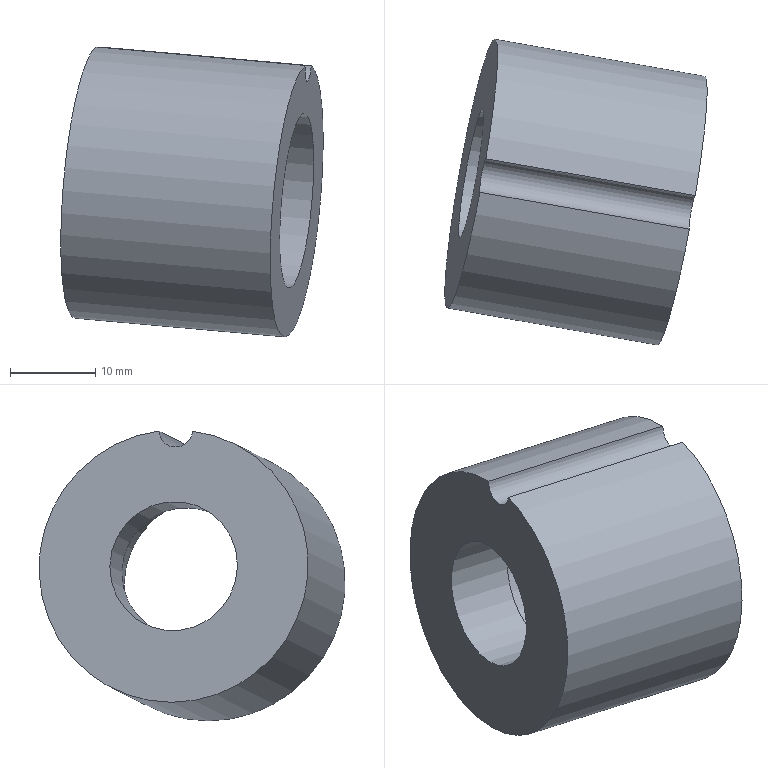Part | NX | features solid 2 | 1 solid | 7 faces | box 30.725 x 35.842 x 33.933 mm | volume 12839 mm3 | cylinder 4 | plane 3 | commonest cylinder face diameters 4 x1 15.18 x1 20.6 x1 32 x1
STEP:
#1=CARTESIAN_POINT('',(580.569,-29.119,46.703));
#2=VERTEX_POINT('',#1);
#3=CARTESIAN_POINT('',(579.875,-33.05,46.703));
#4=VERTEX_POINT('',#3);
#5=CARTESIAN_POINT('',(580.233,-31.086,46.827));
#6=DIRECTION('',(-0.9811,0.173,0.08716));
#7=DIRECTION('',(0.1736,0.9848,0.));
#8=AXIS2_PLACEMENT_3D('',#5,#6,#7);
#9=CIRCLE('',#8,2.);
#10=EDGE_CURVE('',#2,#4,#9,.T.);
#11=ORIENTED_EDGE('',*,*,#10,.F.);
#12=CARTESIAN_POINT('',(578.86,-30.844,30.888));
#13=DIRECTION('',(-0.9811,0.173,0.08716));
#14=DIRECTION('',(0.1736,0.9848,0.));
#15=AXIS2_PLACEMENT_3D('',#12,#13,#14);
#16=CIRCLE('',#15,16.);
#17=EDGE_CURVE('',#2,#4,#16,.T.);
#18=ORIENTED_EDGE('',*,*,#17,.T.);
#19=EDGE_LOOP('',(#11,#18));
#20=FACE_BOUND('',#19,.T.);
#21=CARTESIAN_POINT('',(580.178,-23.369,30.888));
#22=VERTEX_POINT('',#21);
#23=CARTESIAN_POINT('',(578.86,-30.844,30.888));
#24=DIRECTION('',(-0.9811,0.173,0.08716));
#25=DIRECTION('',(0.1736,0.9848,0.));
#26=AXIS2_PLACEMENT_3D('',#23,#24,#25);
#27=CIRCLE('',#26,7.59);
#28=EDGE_CURVE('',#22,#22,#27,.T.);
#29=ORIENTED_EDGE('',*,*,#28,.F.);
#30=EDGE_LOOP('',(#29));
#31=FACE_BOUND('',#30,.T.);
#32=CARTESIAN_POINT('',(578.86,-30.844,30.888));
#33=DIRECTION('',(-0.9811,0.173,0.08716));
#34=DIRECTION('',(-0.1736,-0.9848,0.));
#35=AXIS2_PLACEMENT_3D('',#32,#33,#34);
#36=PLANE('',#35);
#37=ADVANCED_FACE('',(#20,#31),#36,.T.);
#38=CARTESIAN_POINT('',(604.402,-37.375,44.524));
#39=VERTEX_POINT('',#38);
#40=CARTESIAN_POINT('',(605.095,-33.443,44.524));
#41=VERTEX_POINT('',#40);
#42=CARTESIAN_POINT('',(604.759,-35.411,44.649));
#43=DIRECTION('',(0.9811,-0.173,-0.08716));
#44=DIRECTION('',(-0.1736,-0.9848,0.));
#45=AXIS2_PLACEMENT_3D('',#42,#43,#44);
#46=CIRCLE('',#45,2.);
#47=EDGE_CURVE('',#39,#41,#46,.T.);
#48=ORIENTED_EDGE('',*,*,#47,.F.);
#49=CARTESIAN_POINT('',(603.386,-35.169,28.709));
#50=DIRECTION('',(0.9811,-0.173,-0.08716));
#51=DIRECTION('',(-0.1736,-0.9848,0.));
#52=AXIS2_PLACEMENT_3D('',#49,#50,#51);
#53=CIRCLE('',#52,16.);
#54=EDGE_CURVE('',#39,#41,#53,.T.);
#55=ORIENTED_EDGE('',*,*,#54,.T.);
#56=EDGE_LOOP('',(#48,#55));
#57=FACE_BOUND('',#56,.T.);
#58=CARTESIAN_POINT('',(601.597,-45.312,28.709));
#59=VERTEX_POINT('',#58);
#60=CARTESIAN_POINT('',(603.386,-35.169,28.709));
#61=DIRECTION('',(0.9811,-0.173,-0.08716));
#62=DIRECTION('',(-0.1736,-0.9848,0.));
#63=AXIS2_PLACEMENT_3D('',#60,#61,#62);
#64=CIRCLE('',#63,10.3);
#65=EDGE_CURVE('',#59,#59,#64,.T.);
#66=ORIENTED_EDGE('',*,*,#65,.F.);
#67=EDGE_LOOP('',(#66));
#68=FACE_BOUND('',#67,.T.);
#69=CARTESIAN_POINT('',(603.386,-35.169,28.709));
#70=DIRECTION('',(0.9811,-0.173,-0.08716));
#71=DIRECTION('',(0.1736,0.9848,0.));
#72=AXIS2_PLACEMENT_3D('',#69,#70,#71);
#73=PLANE('',#72);
#74=ADVANCED_FACE('',(#57,#68),#73,.T.);
#75=CARTESIAN_POINT('',(592.139,-35.212,45.614));
#76=DIRECTION('',(-0.9811,0.173,0.08716));
#77=VECTOR('',#76,1000.);
#78=LINE('',#75,#77);
#79=EDGE_CURVE('',#39,#4,#78,.T.);
#80=ORIENTED_EDGE('',*,*,#79,.T.);
#81=ORIENTED_EDGE('',*,*,#17,.F.);
#82=CARTESIAN_POINT('',(592.832,-31.281,45.614));
#83=DIRECTION('',(-0.9811,0.173,0.08716));
#84=VECTOR('',#83,1000.);
#85=LINE('',#82,#84);
#86=EDGE_CURVE('',#2,#41,#85,.F.);
#87=ORIENTED_EDGE('',*,*,#86,.T.);
#88=ORIENTED_EDGE('',*,*,#54,.F.);
#89=EDGE_LOOP('',(#80,#81,#87,#88));
#90=FACE_BOUND('',#89,.T.);
#91=CARTESIAN_POINT('',(603.386,-35.169,28.709));
#92=DIRECTION('',(-0.9811,0.173,0.08716));
#93=DIRECTION('',(-0.1736,-0.9848,0.));
#94=AXIS2_PLACEMENT_3D('',#91,#92,#93);
#95=CYLINDRICAL_SURFACE('',#94,16.);
#96=ADVANCED_FACE('',(#90),#95,.T.);
#97=CARTESIAN_POINT('',(585.39,-39.703,30.191));
#98=VERTEX_POINT('',#97);
#99=CARTESIAN_POINT('',(586.708,-32.228,30.191));
#100=DIRECTION('',(0.9811,-0.173,-0.08716));
#101=DIRECTION('',(-0.1736,-0.9848,0.));
#102=AXIS2_PLACEMENT_3D('',#99,#100,#101);
#103=CIRCLE('',#102,7.59);
#104=EDGE_CURVE('',#98,#98,#103,.T.);
#105=ORIENTED_EDGE('',*,*,#104,.F.);
#106=EDGE_LOOP('',(#105));
#107=FACE_BOUND('',#106,.T.);
#108=CARTESIAN_POINT('',(588.497,-22.084,30.191));
#109=VERTEX_POINT('',#108);
#110=CARTESIAN_POINT('',(586.708,-32.228,30.191));
#111=DIRECTION('',(-0.9811,0.173,0.08716));
#112=DIRECTION('',(0.1736,0.9848,0.));
#113=AXIS2_PLACEMENT_3D('',#110,#111,#112);
#114=CIRCLE('',#113,10.3);
#115=EDGE_CURVE('',#109,#109,#114,.T.);
#116=ORIENTED_EDGE('',*,*,#115,.F.);
#117=EDGE_LOOP('',(#116));
#118=FACE_BOUND('',#117,.T.);
#119=CARTESIAN_POINT('',(586.708,-32.228,30.191));
#120=DIRECTION('',(-0.9811,0.173,0.08716));
#121=DIRECTION('',(-0.1736,-0.9848,0.));
#122=AXIS2_PLACEMENT_3D('',#119,#120,#121);
#123=PLANE('',#122);
#124=ADVANCED_FACE('',(#107,#118),#123,.F.);
#125=ORIENTED_EDGE('',*,*,#115,.T.);
#126=EDGE_LOOP('',(#125));
#127=FACE_BOUND('',#126,.T.);
#128=ORIENTED_EDGE('',*,*,#65,.T.);
#129=EDGE_LOOP('',(#128));
#130=FACE_BOUND('',#129,.T.);
#131=CARTESIAN_POINT('',(603.386,-35.169,28.709));
#132=DIRECTION('',(-0.9811,0.173,0.08716));
#133=DIRECTION('',(-0.1736,-0.9848,0.));
#134=AXIS2_PLACEMENT_3D('',#131,#132,#133);
#135=CYLINDRICAL_SURFACE('',#134,10.3);
#136=ADVANCED_FACE('',(#127,#130),#135,.F.);
#137=ORIENTED_EDGE('',*,*,#28,.T.);
#138=EDGE_LOOP('',(#137));
#139=FACE_BOUND('',#138,.T.);
#140=ORIENTED_EDGE('',*,*,#104,.T.);
#141=EDGE_LOOP('',(#140));
#142=FACE_BOUND('',#141,.T.);
#143=CARTESIAN_POINT('',(586.708,-32.228,30.191));
#144=DIRECTION('',(-0.9811,0.173,0.08716));
#145=DIRECTION('',(-0.1736,-0.9848,0.));
#146=AXIS2_PLACEMENT_3D('',#143,#144,#145);
#147=CYLINDRICAL_SURFACE('',#146,7.59);
#148=ADVANCED_FACE('',(#139,#142),#147,.F.);
#149=ORIENTED_EDGE('',*,*,#79,.F.);
#150=ORIENTED_EDGE('',*,*,#47,.T.);
#151=ORIENTED_EDGE('',*,*,#86,.F.);
#152=ORIENTED_EDGE('',*,*,#10,.T.);
#153=EDGE_LOOP('',(#149,#150,#151,#152));
#154=FACE_BOUND('',#153,.T.);
#155=CARTESIAN_POINT('',(604.759,-35.411,44.649));
#156=DIRECTION('',(-0.9811,0.173,0.08716));
#157=DIRECTION('',(-0.1736,-0.9848,0.));
#158=AXIS2_PLACEMENT_3D('',#155,#156,#157);
#159=CYLINDRICAL_SURFACE('',#158,2.);
#160=ADVANCED_FACE('',(#154),#159,.F.);
#161=CLOSED_SHELL('',(#37,#74,#96,#124,#136,#148,#160));
#162=MANIFOLD_SOLID_BREP('',#161);
#163=(LENGTH_UNIT()NAMED_UNIT(*)SI_UNIT(.MILLI.,.METRE.));
#164=UNCERTAINTY_MEASURE_WITH_UNIT(LENGTH_MEASURE(0.00001),#163,'','');
#165=(NAMED_UNIT(*)PLANE_ANGLE_UNIT()SI_UNIT($,.RADIAN.));
#166=(NAMED_UNIT(*)SI_UNIT($,.STERADIAN.)SOLID_ANGLE_UNIT());
#167=(GEOMETRIC_REPRESENTATION_CONTEXT(3)GLOBAL_UNCERTAINTY_ASSIGNED_CONTEXT((#164))GLOBAL_UNIT_ASSIGNED_CONTEXT((#163,#165,#166))REPRESENTATION_CONTEXT('',''));
#168=ADVANCED_BREP_SHAPE_REPRESENTATION('',(#162),#167);